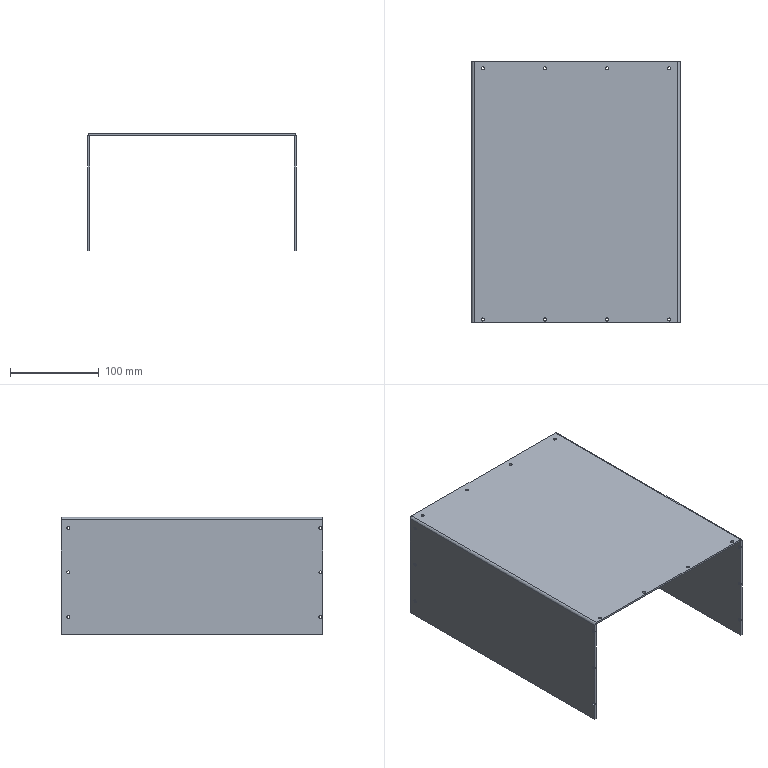Part | STEP file | GLSJ-10-34 | 1 solid | 62 faces | box 234 x 294 x 132 mm | volume 289211 mm3 | cylinder 44 | plane 18 | commonest cylinder face diameters 3.5 x40 1.473 x2 5.473 x2